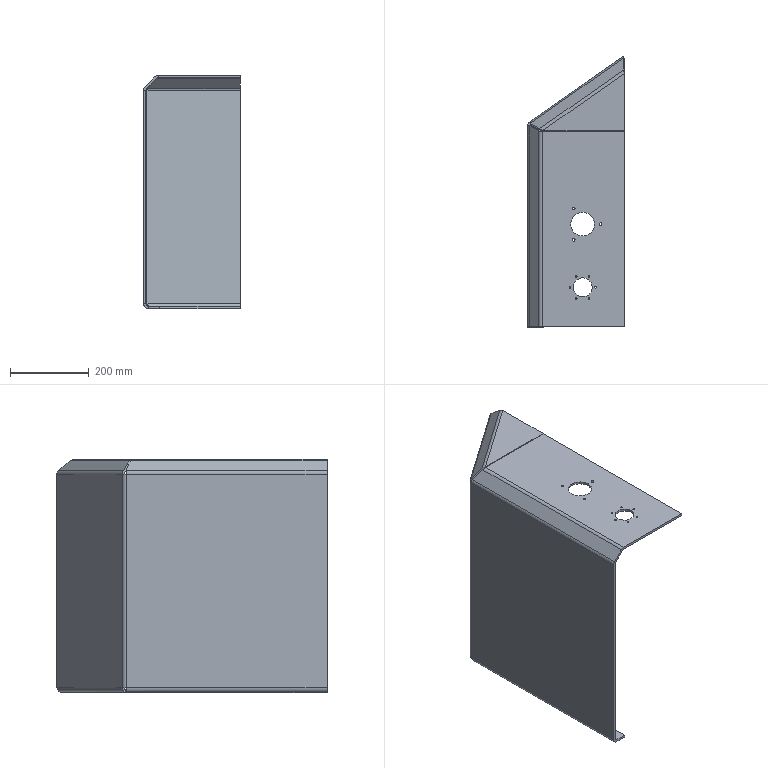Part | SolidWorks | features ICE 4, EdgeFlange 3, HoleWzd 2, FlatPattern 1, SMBaseFlange 1, SheetMetal 1 | 1 solid | 95 faces | box 244.999 x 684.15 x 590 mm | volume 3721294 mm3 | plane 45 | cylinder 44 | spline 6 | commonest cylinder face diameters 4.2 x12 8.5 x8 12 x7 24 x7 6.8 x6 48 x2